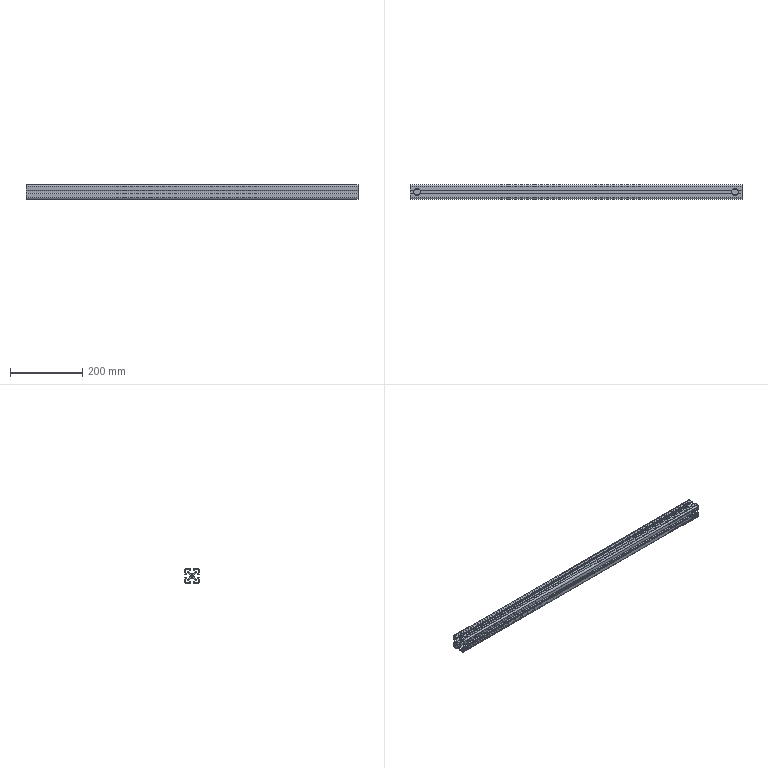Part | STEP file | MK-8-4040C-L-04 profile 4040C standard 920mm | 1 solid | 316 faces | box 920 x 40 x 40 mm | volume 435718 mm3 | cylinder 166 | plane 150 | commonest cylinder face diameters 0.6 x62 2 x36 4 x24 0.4 x16 19 x16 6 x4